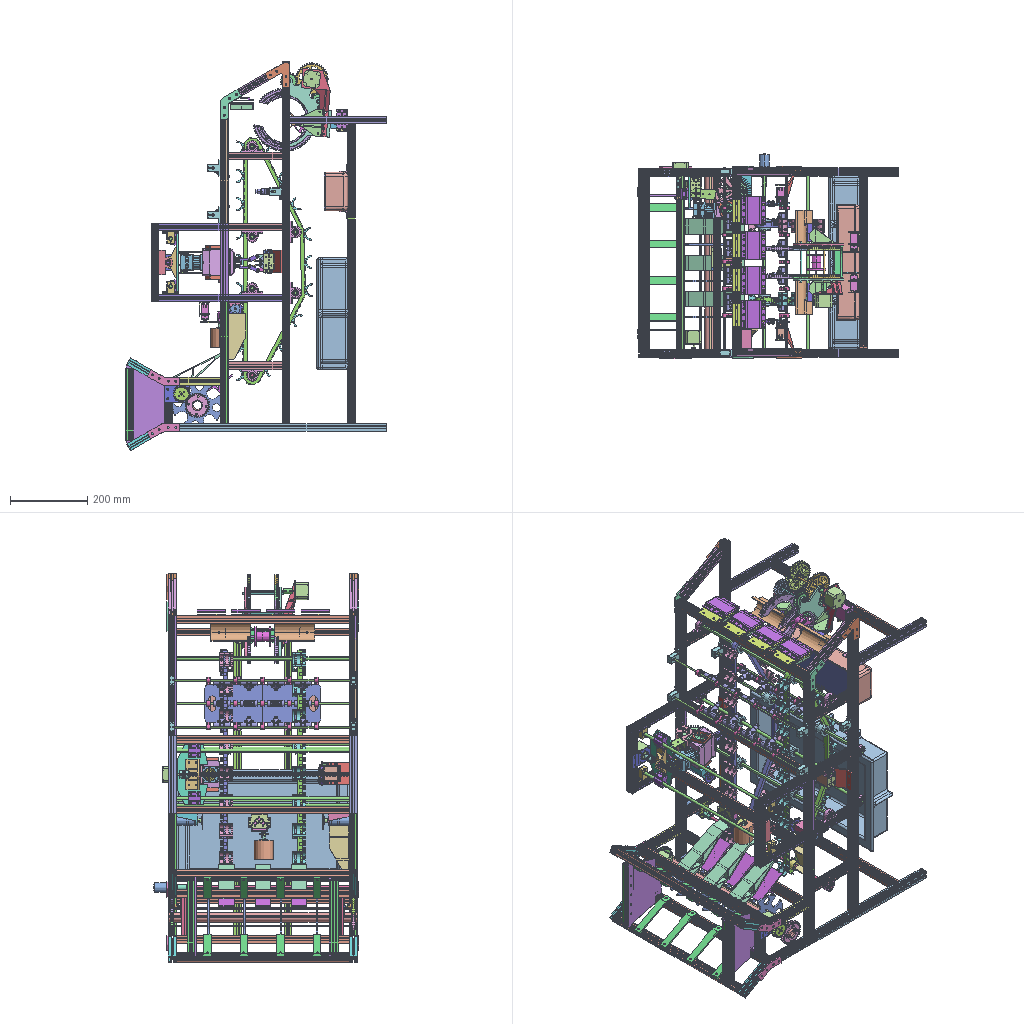Assembly | STEP file | 130 different items | 376 placed | box 676 x 533 x 1010 mm
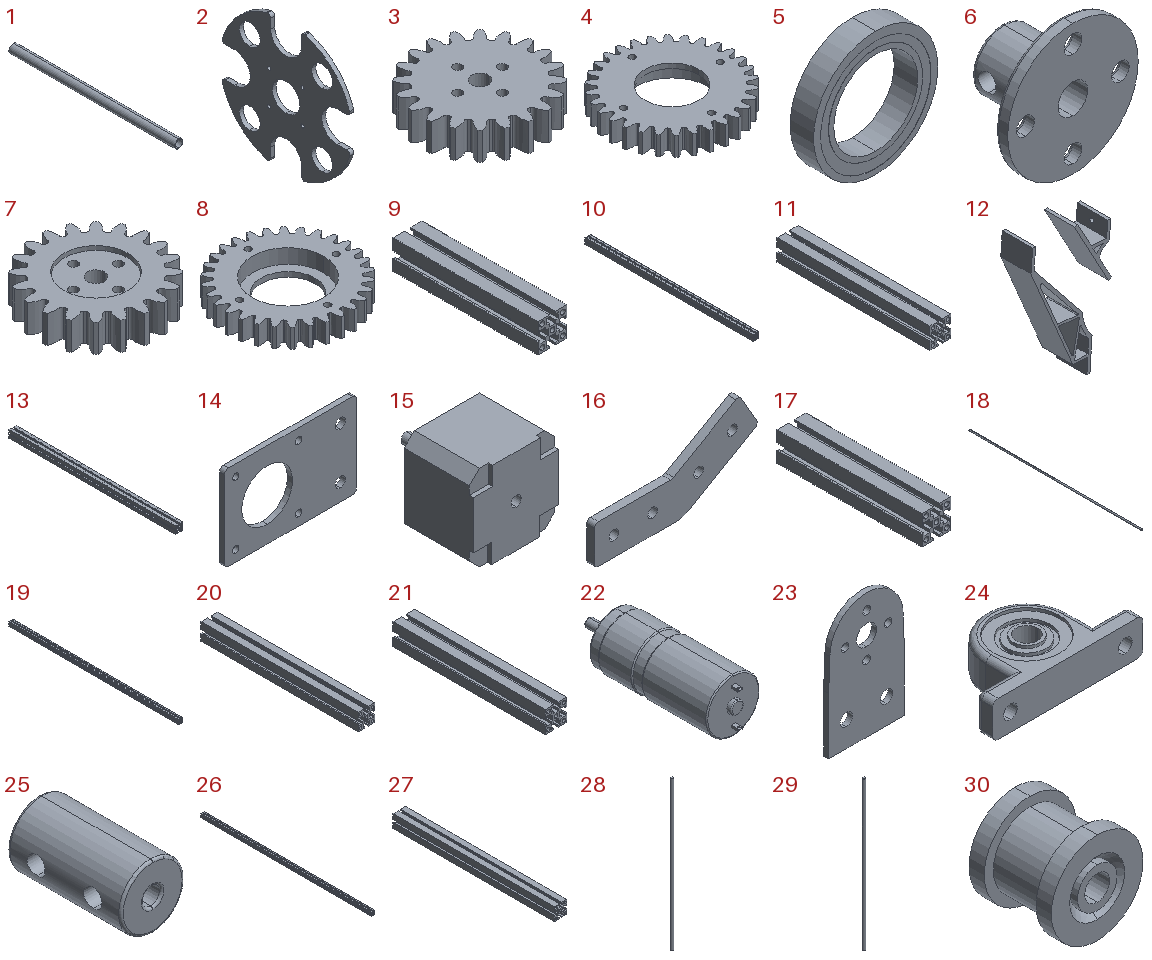Parts list (item | name | quantity | parent item | size | volume):
1 | Central air duct | x1 | - | 25 x 490 x 25 mm | 70811 mm3
2 | Chuck wheel | x4 | - | 4 x 124.659 x 124.659 mm | 32758 mm3
3 | Chuck drive gear | x1 | - | 43.654 x 43.654 x 10 mm | 11238 mm3
4 | Chuck gear | x1 | - | 64 x 63.787 x 10 mm | 17915 mm3
5 | Wheel bearing | x2 | - | 37 x 7 x 37 mm | 4043 mm3
6 | Flange coupling 5 | x2 | - | 22 x 12 x 22 mm | 1230 mm3
7 | Mirror chuck drive gear | x1 | - | 43.654 x 43.654 x 10 mm | 11238 mm3
8 | Mirror chuck gear | x1 | - | 64 x 63.787 x 10 mm | 17915 mm3
9 | 20 aluminium profile longitudinal 1 | x2 | - | 20 x 100 x 20 mm | 17778 mm3
10 | 20 aluminium profile vertical 1 | x2 | - | 20 x 575 x 20 mm | 102223 mm3
11 | 20 aluminium profile vertical 2 | x2 | - | 20 x 145 x 20 mm | 25778 mm3
12 | Chuck limit ring | x3 | - | 105.924 x 40 x 181.464 mm | 85930 mm3
13 | 20 aluminium profile transverse 2 | x10 | - | 20 x 450 x 20 mm | 80001 mm3
14 | 42 stepper aluminium flat bracket | x3 | - | 65 x 2.5 x 42 mm | 5411 mm3
15 | 42 stepper motor 34 | x4 | - | 42 x 54 x 42 mm | 57864 mm3
16 | 150-degree side frame | x4 | - | 83.909 x 4 x 39.268 mm | 6499 mm3
17 | 20 aluminium profile diagonal 1 | x4 | - | 20 x 100 x 20 mm | 17778 mm3
18 | Gear shaft | x4 | - | 4 x 491 x 4 mm | 6170 mm3
19 | 20 aluminium profile longitudinal 1 | x2 | - | 20 x 830 x 20 mm | 147557 mm3
20 | 20 aluminium profile longitudinal 2 | x2 | - | 20 x 186 x 20 mm | 33067 mm3
21 | 20 aluminium profile vertical 1 | x6 | - | 20 x 140 x 20 mm | 24889 mm3
22 | 370 straight motor | x3 | - | 25 x 71.68 x 25 mm | 27082 mm3
23 | Smooth shaft 370 bracket | x1 | - | 30 x 2 x 49.5 mm | 2512 mm3
24 | U-type bearing support 8 | x11 | - | 55 x 30 x 13 mm | 10419 mm3
25 | 48 rigid coupling | x1 | - | 14 x 25 x 14 mm | 2952 mm3
26 | 20 aluminium profile longitudinal 3 | x2 | - | 20 x 940 x 20 mm | 167113 mm3
27 | 20 aluminium profile vertical 2 | x2 | - | 20 x 250 x 20 mm | 44445 mm3
28 | Sprocket 1 shaft | x7 | - | 8 x 8 x 490 mm | 24630 mm3
29 | Sprocket 2 shaft | x1 | - | 8 x 8 x 480 mm | 24127 mm3
30 | B drag chain wheel | x10 | - | 30 x 27 x 30 mm | 13045 mm3
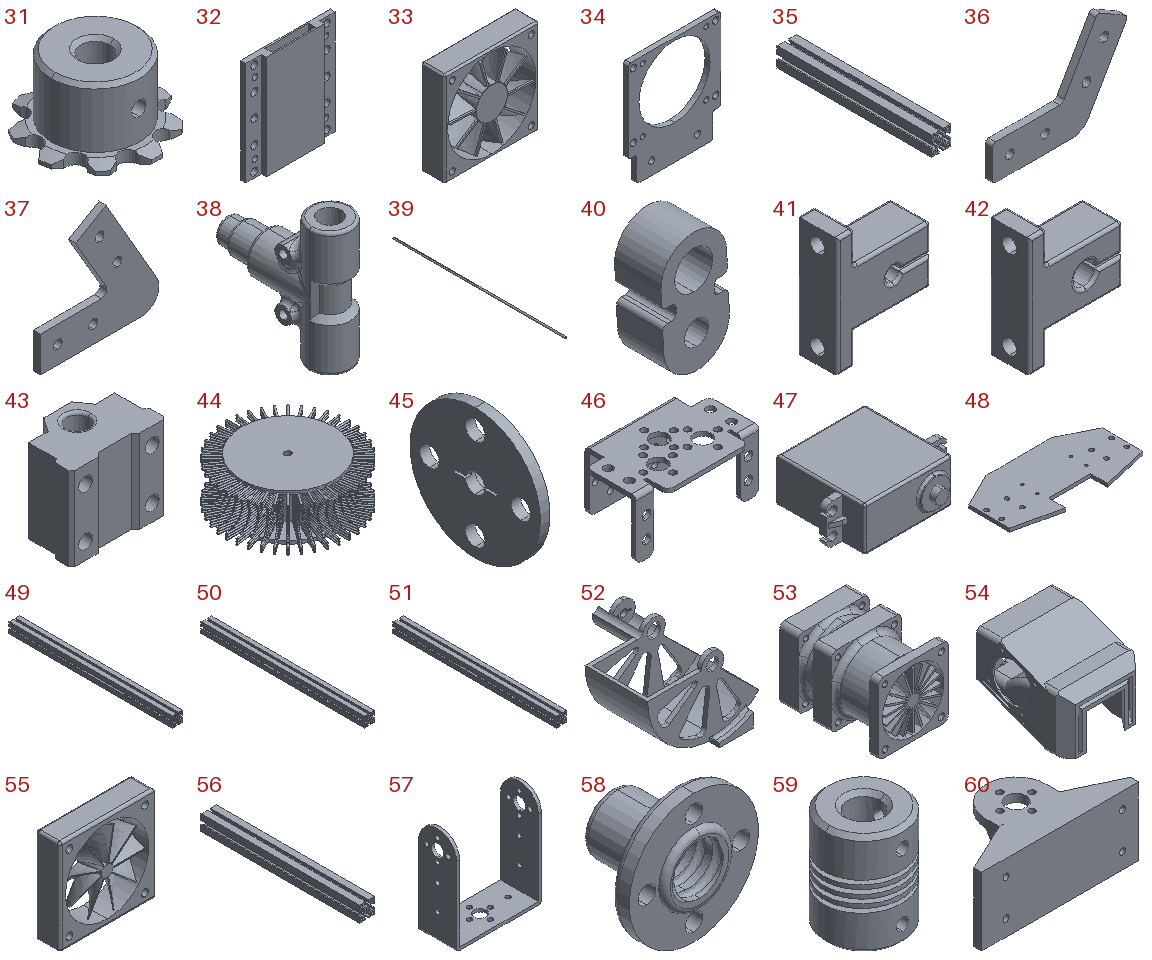31 | Sprocket | x2 | - | 33.749 x 33.304 x 20 mm | 8415 mm3
32 | Heating module 60 low | x4 | - | 63 x 7 x 73 mm | 14494 mm3
33 | Fan 60 | x4 | - | 60 x 15 x 60 mm | 65760 mm3
34 | Drying connection frame | x4 | - | 73 x 4 x 85 mm | 13236 mm3
35 | 20 aluminium profile diagonal 2 | x2 | - | 20 x 160 x 20 mm | 28445 mm3
36 | 120-degree side frame | x2 | - | 76.588 x 4 x 53.909 mm | 6976 mm3
37 | 60-degree side frame | x2 | - | 67.321 x 4 x 64.641 mm | 8608 mm3
38 | Water-bath atomizer head | x12 | - | 15 x 44.7 x 45 mm | 9906 mm3
39 | Cleaning nozzle shaft | x3 | - | 5 x 490 x 5 mm | 9621 mm3
40 | Rotating slot | x15 | - | 14.79 x 10 x 26.2 mm | 2369 mm3
41 | T-type support 5(D) | x6 | - | 32.8 x 14 x 42 mm | 10262 mm3
42 | T-type support 8 | x4 | - | 32.8 x 14 x 42 mm | 9873 mm3
43 | Slider 8 | x2 | - | 34 x 22 x 30 mm | 14928 mm3
44 | Wheel brush | x1 | - | 80 x 80 x 30 mm | 40010 mm3
45 | Large servo disc | x4 | - | 3.5 x 20 x 20 mm | 468.717 mm3
46 | Multifunction bracket | x5 | - | 58 x 37.5 x 28 mm | 5928 mm3
47 | Servo single shaft | x5 | in SW alloy mechanical claw | 55 x 44.5 x 20 mm | 32938 mm3
48 | Sliding plate | x1 | - | 158 x 80 x 4 mm | 40027 mm3
49 | 20 aluminium profile longitudinal 4 | x2 | - | 20 x 310 x 20 mm | 55112 mm3
50 | 20 aluminium profile vertical 6 | x4 | - | 20 x 320 x 20 mm | 56889 mm3
51 | 20 aluminium profile longitudinal 5 | x2 | - | 20 x 316 x 20 mm | 56178 mm3
52 | Peel friction cover | x1 | - | 81.568 x 81 x 58.817 mm | 32383 mm3
53 | Vortex fan 40 | x1 | - | 40 x 56 x 40 mm | 33950 mm3
54 | U-type air nozzle | x1 | - | 70 x 80.5 x 65.068 mm | 54553 mm3
55 | Fan 40 | x2 | - | 40 x 10 x 40 mm | 6606 mm3
56 | 20 aluminium profile longitudinal 6 | x2 | - | 20 x 204 x 20 mm | 36267 mm3
57 | U long bracket | x1 | - | 56 x 25 x 64.5 mm | 8183 mm3
58 | Lead screw nut 8 | x1 | - | 22 x 15 x 22 mm | 1124 mm3
59 | 58 flexible coupling | x1 | - | 19 x 19 x 25 mm | 4870 mm3
60 | Lead screw push block | x1 | - | 78 x 37 x 34 mm | 16349 mm3
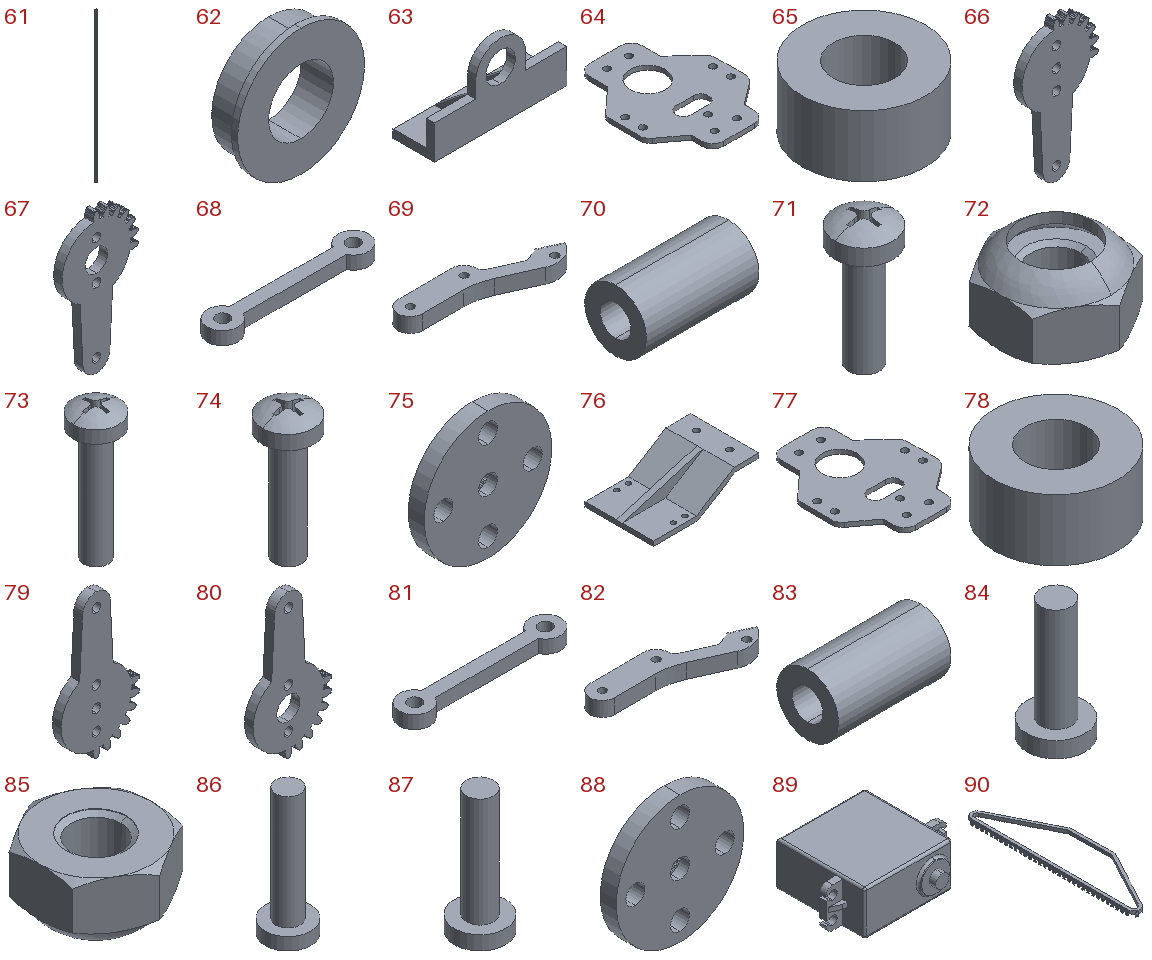61 | Lead screw 1 | x1 | - | 8 x 8 x 450 mm | 16512 mm3
62 | Bearing 814 | x1 | - | 15.6 x 4 x 15.6 mm | 433.486 mm3
63 | Lead screw bearing sleeve | x1 | - | 64.2 x 20 x 36.1 mm | 9790 mm3
64 | Gripper (new)_1 | x1 | in SW alloy mechanical claw | 48 x 61 x 2 mm | 3505 mm3
65 | Small washer_1 | x3 | in SW alloy mechanical claw | 6 x 6 x 3 mm | 63.617 mm3
66 | Claw gear 2 | x1 | in SW alloy mechanical claw | 27.091 x 3 x 49.757 mm | 2108 mm3
67 | Claw gear_1 | x1 | in SW alloy mechanical claw | 27.091 x 3 x 49.757 mm | 1979 mm3
68 | Small crossbar_1 | x2 | in SW alloy mechanical claw | 37 x 7 x 3 mm | 397.481 mm3
69 | Long rod_1 | x2 | in SW alloy mechanical claw | 59.158 x 19.551 x 6 mm | 2724 mm3
70 | Stud_1 | x4 | in SW alloy mechanical claw | 11 x 6 x 6 mm | 233.263 mm3
71 | GB818-M3X10-ZN-4.8_1 | x2 | in SW alloy mechanical claw | 5.6 x 5.6 x 12.376 mm | 116.575 mm3
72 | GB6170-M3 (self-locking)_1 | x9 | in SW alloy mechanical claw | 5.5 x 6.351 x 3.382 mm | 56.307 mm3
73 | GB818-M3X14-ZN-4.8_1 | x6 | in SW alloy mechanical claw | 5.6 x 5.6 x 16.376 mm | 144.849 mm3
74 | GB818-M3X12-ZN-4.8_1 | x1 | in SW alloy mechanical claw | 5.6 x 5.6 x 14.376 mm | 130.712 mm3
75 | Metal main rudder disc | x1 | in SW alloy mechanical claw | 20 x 4.5 x 20 mm | 750.526 mm3
76 | Mechanical claw bracket | x2 | - | 90 x 58 x 24 mm | 23689 mm3
77 | Mirror gripper (new)_1 | x1 | in MirrorSW alloy mechanical claw | 48 x 61 x 2 mm | 3505 mm3
78 | Mirror small washer_1 | x3 | in MirrorSW alloy mechanical claw | 6 x 6 x 3 mm | 63.617 mm3
79 | Mirror claw gear 2 | x1 | in MirrorSW alloy mechanical claw | 27.091 x 3 x 49.757 mm | 2108 mm3
80 | Mirror claw gear_1 | x1 | in MirrorSW alloy mechanical claw | 27.091 x 3 x 49.757 mm | 1979 mm3
81 | Mirror small crossbar_1 | x2 | in MirrorSW alloy mechanical claw | 37 x 7 x 3 mm | 397.481 mm3
82 | Mirror long rod_1 | x2 | in MirrorSW alloy mechanical claw | 59.158 x 19.551 x 6 mm | 2724 mm3
83 | Mirror stud_1 | x4 | in MirrorSW alloy mechanical claw | 11 x 6 x 6 mm | 233.263 mm3
84 | MirrorGB818-M3X10-ZN-4.8_1 | x2 | in MirrorSW alloy mechanical claw | 5.6 x 5.6 x 12.376 mm | 116.575 mm3
85 | MirrorGB6170-M3 (self-locking)_1 | x9 | in MirrorSW alloy mechanical claw | 5.5 x 6.351 x 3.382 mm | 56.307 mm3
86 | MirrorGB818-M3X14-ZN-4.8_1 | x6 | in MirrorSW alloy mechanical claw | 5.6 x 5.6 x 16.376 mm | 144.849 mm3
87 | MirrorGB818-M3X12-ZN-4.8_1 | x1 | in MirrorSW alloy mechanical claw | 5.6 x 5.6 x 14.376 mm | 130.712 mm3
88 | Mirror metal main rudder disc | x1 | in MirrorSW alloy mechanical claw | 20 x 4.5 x 20 mm | 750.526 mm3
89 | Mirror servo single shaft | x1 | in MirrorSW alloy mechanical claw | 55 x 44.5 x 20 mm | 32938 mm3
90 | Belt 1 | x1 | - | 163.112 x 641.3 x 20 mm | 175468 mm3
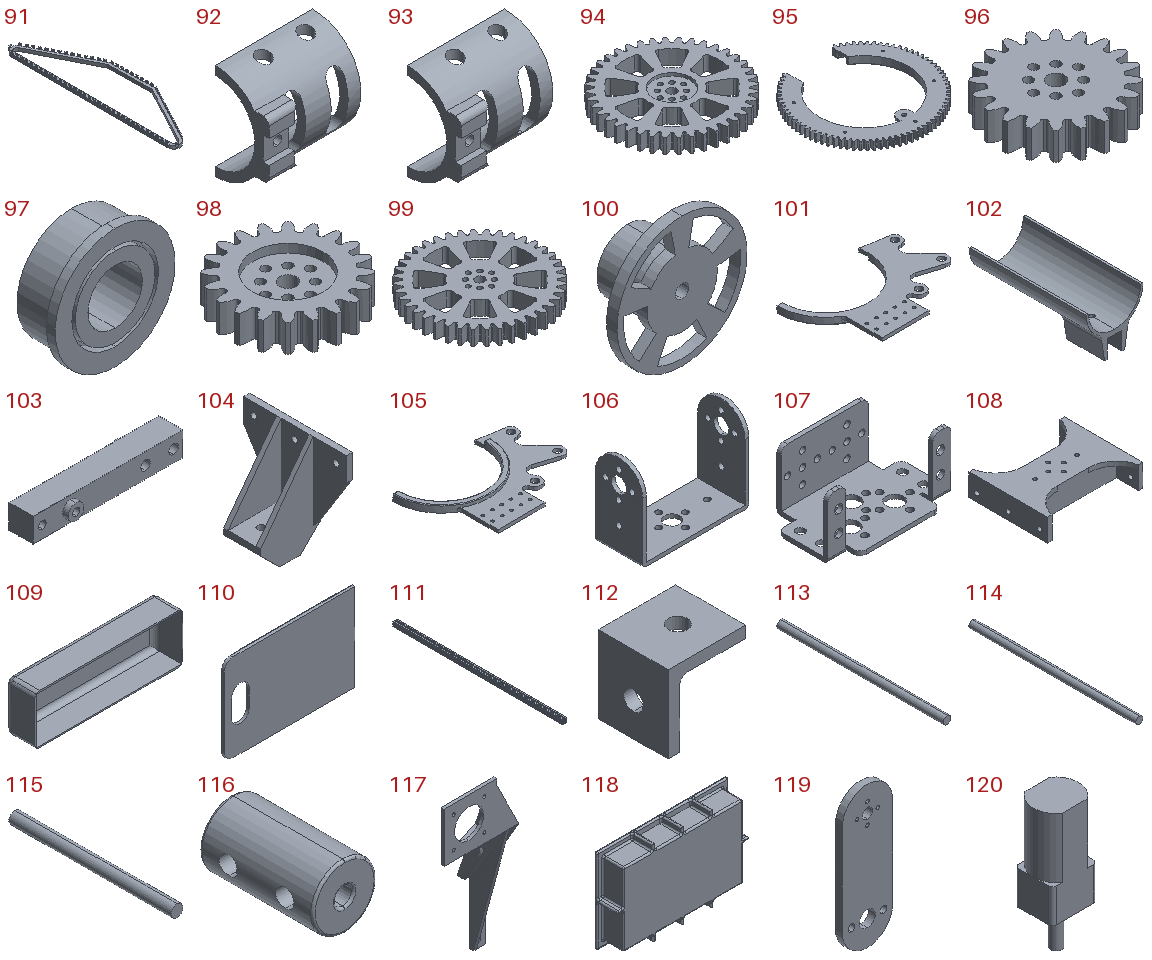91 | Mirror belt 1 | x1 | - | 163.112 x 641.3 x 20 mm | 175468 mm3
92 | Chain frame | x18 | - | 34.45 x 19 x 34 mm | 4420 mm3
93 | Mirror chain frame | x18 | - | 34.45 x 19 x 34 mm | 4420 mm3
94 | FD gear 40 | x1 | - | 83.847 x 83.847 x 10 mm | 32005 mm3
95 | Packing half-gear | x2 | - | 163.929 x 156.763 x 10 mm | 60681 mm3
96 | FD gear 20 | x2 | - | 43.654 x 43.654 x 10 mm | 10262 mm3
97 | Flange bearing 5104 | x6 | - | 11 x 4 x 11 mm | 233.729 mm3
98 | MirrorFD gear 20 | x2 | - | 43.654 x 43.654 x 10 mm | 10262 mm3
99 | MirrorFD gear 40 | x1 | - | 83.847 x 83.847 x 10 mm | 32005 mm3
100 | Packing half-frame | x2 | - | 50 x 21 x 50 mm | 8229 mm3
101 | Half-gear guide groove revised | x1 | - | 193.874 x 133 x 10.2 mm | 53575 mm3
102 | Weighing slot | x2 | - | 50 x 103.5 x 42.709 mm | 22376 mm3
103 | Weighing module | x2 | - | 80 x 18.8 x 12.8 mm | 12498 mm3
104 | Weighing fixed frame | x2 | - | 40 x 70 x 65.291 mm | 23281 mm3
105 | Mirror half-gear guide groove revised | x1 | - | 193.874 x 133 x 10.2 mm | 53575 mm3
106 | U short bracket | x1 | - | 56 x 25 x 44.5 mm | 6211 mm3
107 | Mirror multifunction bracket | x1 | - | 58 x 37.5 x 28 mm | 5928 mm3
108 | Servo connection frame | x1 | - | 85 x 70 x 20 mm | 29316 mm3
109 | 301 water tank | x1 | - | 300 x 58 x 100 mm | 214812 mm3
110 | 301 water tank cover | x2 | - | 150 x 6 x 100 mm | 46035 mm3
111 | 20 aluminium profile longitudinal 7 | x2 | - | 20 x 778 x 20 mm | 138312 mm3
112 | 20 angle bracket flat | x8 | - | 20 x 18 x 20 mm | 1896 mm3
113 | Rear shaft short | x2 | - | 5 x 106 x 5 mm | 2081 mm3
114 | Rear shaft long | x1 | - | 5 x 116 x 5 mm | 2278 mm3
115 | Rear winding spool | x1 | - | 5 x 68 x 5 mm | 1335 mm3
116 | 55 rigid coupling | x1 | - | 14 x 25 x 14 mm | 3316 mm3
117 | Rear stepper bracket | x1 | - | 75 x 37 x 171.474 mm | 24600 mm3
118 | Basket 1 | x1 | - | 450 x 80 x 290 mm | 2294003 mm3
119 | Dial wheel bracket | x1 | - | 22 x 3 x 62 mm | 3552 mm3
120 | N201 | x2 | - | 12 x 10 x 35 mm | 2772 mm3
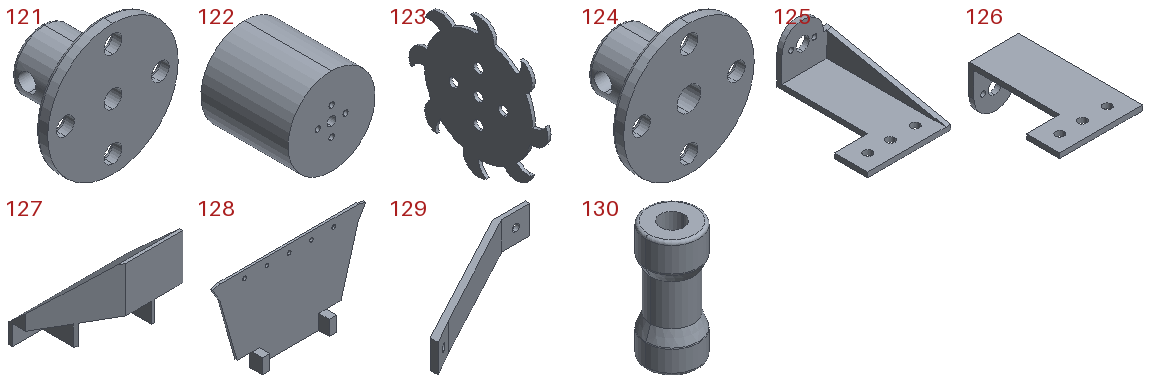121 | Flange coupling 3 | x1 | - | 22 x 12 x 22 mm | 1380 mm3
122 | Dial wheel | x1 | - | 50 x 50 x 50 mm | 41621 mm3
123 | Cutting knife | x2 | - | 1 x 45 x 45 mm | 1128 mm3
124 | Flange coupling 4 | x2 | - | 22 x 12 x 22 mm | 1314 mm3
125 | Cutting motor bracket | x1 | - | 50 x 74.62 x 30.335 mm | 11204 mm3
126 | Mirror cutting motor bracket | x1 | - | 50 x 74.62 x 30.335 mm | 11204 mm3
127 | Top plate | x1 | - | 120 x 53 x 65 mm | 56002 mm3
128 | Bin side panel | x2 | - | 206.163 x 17 x 120.782 mm | 62585 mm3
129 | Front frame | x8 | - | 118.103 x 56.081 x 20 mm | 10734 mm3
130 | Brass coupling 3-4 | x1 | - | 9 x 9 x 20 mm | 848.219 mm3
Placements (level | parent | child | x y z in mm | rotation matrix by rows), first 264 of 378 lines:
1 | subassembly 2 | Central air duct | -58.969 -295.759 -262.917 | 0.04399 0 -0.999 0 1 0 0.999 0 0.04399
1 | subassembly 2 | Chuck wheel | -58.969 -152.758 -262.917 | 0 0.6192 0.7852 -1 0 0 0 -0.7852 0.6192
1 | subassembly 2 | Chuck drive gear | -99.969 -526.259 -233.434 | -0.6467 -0.7627 0 0 0 -1 0.7627 -0.6467 -0
1 | subassembly 2 | Chuck gear | -58.969 -526.259 -262.917 | -0.02036 0.9998 0 0 0 -1 -0.9998 -0.02036 -0
1 | subassembly 2 | Wheel bearing | -58.969 -530.259 -262.917 | 1 0 0 0 1 0 0 0 1
1 | subassembly 2 | Flange coupling 5 | -99.969 -527.759 -233.434 | 0.6467 0 0.7627 0 1 0 -0.7627 0 0.6467
1 | subassembly 2 | Chuck wheel | -58.969 -438.759 -262.917 | 0 0.6192 -0.7852 1 0 0 0 -0.7852 -0.6192
1 | subassembly 2 | Mirror chuck drive gear | -99.969 -65.258 -233.434 | -0.6467 -0.7627 0 0 0 -1 0.7627 -0.6467 -0
1 | subassembly 2 | Flange coupling 5 | -99.969 -63.758 -233.434 | 0.6467 0 -0.7627 0 -1 0 -0.7627 0 -0.6467
1 | subassembly 2 | Mirror chuck gear | -58.969 -65.258 -262.917 | -0.02036 0.9998 0 0 0 -1 -0.9998 -0.02036 -0
1 | subassembly 2 | Wheel bearing | -58.969 -61.258 -262.917 | -1 0 0 0 -1 0 0 0 1
1 | subassembly 2 | 20 aluminium profile longitudinal 1 | -133.969 -495.759 -210.171 | 1 0 0 0 0 1 0 -1 -0
1 | subassembly 2 | 20 aluminium profile vertical 1 | -143.969 -60.758 -320.171 | 0 1 0 -1 0 0 0 0 1
1 | subassembly 2 | 20 aluminium profile vertical 2 | -143.969 -60.758 -200.171 | 0 1 0 -1 0 0 0 0 1
1 | subassembly 2 | Chuck limit ring | -59.043 -409.759 -261.81 | 0.06683 0 0.9978 0 1 0 -0.9978 0 0.06683
1 | subassembly 2 | 20 aluminium profile transverse 2 | -228.411 -520.759 -153.429 | 0.866 0 0.5 0 1 0 -0.5 0 0.866
1 | subassembly 2 | Chuck limit ring | -59.043 -221.758 -261.81 | 0.06683 0 0.9978 0 1 0 -0.9978 0 0.06683
1 | subassembly 2 | 42 stepper aluminium flat bracket | -111.469 -507.009 -233.434 | -1 0 0 0 -1 0 0 0 1
1 | subassembly 2 | 42 stepper motor 34 | -99.969 -471.759 -233.434 | 1 0 0 0 -1 0 0 0 -1
1 | subassembly 2 | 150-degree side frame | -144.773 -46.758 -330.171 | 0.866 0 0.5 0 -1 0 0.5 0 -0.866
1 | subassembly 2 | 150-degree side frame | -144.773 -50.758 -190.171 | 0.866 0 0.5 0 1 0 -0.5 0 0.866
1 | subassembly 2 | 20 aluminium profile diagonal 1 | -237.071 -60.758 -371.913 | 0 0.866 -0.5 -1 0 0 0 0.5 0.866
1 | subassembly 2 | 20 aluminium profile diagonal 1 | -237.071 -60.758 -148.429 | 0 0.866 0.5 -1 0 0 0 -0.5 0.866
1 | subassembly 2 | 20 aluminium profile transverse 2 | -133.969 -520.759 -320.171 | 1 0 0 0 1 0 0 0 1
1 | subassembly 2 | 20 aluminium profile transverse 2 | -228.411 -520.759 -366.913 | 0.866 0 -0.5 0 1 0 0.5 0 0.866
1 | subassembly 2 | 20 aluminium profile vertical 2 | -143.969 -530.759 -200.171 | 0 1 0 1 0 0 0 0 -1
1 | subassembly 2 | 42 stepper aluminium flat bracket | -111.469 -84.508 -233.434 | -1 0 0 0 1 0 0 0 -1
1 | subassembly 2 | 42 stepper motor 34 | -99.969 -119.758 -233.434 | 1 0 0 0 1 0 0 0 1
1 | subassembly 2 | 20 aluminium profile vertical 1 | -143.969 -530.759 -320.171 | 0 1 0 1 0 0 0 0 -1
1 | subassembly 2 | 20 aluminium profile longitudinal 1 | -133.969 -95.758 -210.171 | 1 0 0 0 0 1 0 -1 0
1 | subassembly 2 | 150-degree side frame | -144.773 -544.759 -190.171 | 0.866 0 0.5 0 1 0 -0.5 0 0.866
1 | subassembly 2 | 20 aluminium profile diagonal 1 | -237.071 -530.759 -148.429 | 0 0.866 -0.5 1 0 0 0 -0.5 -0.866
1 | subassembly 2 | 150-degree side frame | -144.773 -540.759 -330.171 | 0.866 0 0.5 0 -1 0 0.5 0 -0.866
1 | subassembly 2 | 20 aluminium profile diagonal 1 | -237.071 -530.759 -371.913 | 0 0.866 0.5 1 0 0 0 0.5 -0.866
1 | subassembly 2 | 20 aluminium profile transverse 2 | -133.969 -520.759 -200.171 | 1 0 0 0 1 0 0 0 1
1 | subassembly 2 | Gear shaft | -56.269 -541.259 -240.076 | -0.5288 0 0.8488 0 1 0 -0.8488 0 -0.5288
1 | subassembly 2 | Gear shaft | -81.81 -541.259 -260.216 | 0.8488 0 0.5288 0 1 0 -0.5288 0 0.8488
1 | subassembly 2 | Gear shaft | -61.669 -541.259 -285.758 | 0.5288 0 -0.8488 0 1 0 0.8488 0 0.5288
1 | subassembly 2 | Gear shaft | -36.128 -541.259 -265.617 | -0.8488 0 -0.5288 0 1 0 0.5288 0 -0.8488
1 | subassembly 2 | Chuck wheel | -58.969 -246.758 -262.917 | 0 0.6192 0.7852 -1 0 0 0 -0.7852 0.6192
1 | subassembly 2 | Chuck wheel | -58.969 -344.759 -262.917 | 0 0.6192 -0.7852 1 0 0 0 -0.7852 -0.6192
1 | subassembly 2 | Chuck limit ring | -59.043 -315.759 -261.81 | 0.06683 0 0.9978 0 1 0 -0.9978 0 0.06683
1 | subassembly 2 | 20 aluminium profile longitudinal 1 | 11.031 -60.758 519.829 | 0 0 1 -1 0 0 0 -1 0
1 | subassembly 2 | 20 aluminium profile transverse 2 | 11.019 -70.758 -216.604 | -1 0 0 0 -1 0 0 0 1
1 | subassembly 2 | 20 aluminium profile longitudinal 2 | -234.751 -109.758 -167.09 | -1 0 0 0 0 -1 0 -1 -0
1 | subassembly 2 | 20 aluminium profile vertical 1 | 161.031 -60.758 -160.171 | 0 -1 0 1 0 0 0 0 1
1 | subassembly 2 | 370 straight motor | 83.531 -14.959 -185.171 | 1 0 0 0 -1 0 0 0 -1
1 | subassembly 2 | Smooth shaft 370 bracket | 83.531 -70.758 -160.171 | 1 0 0 0 -1 0 0 0 -1
1 | subassembly 2 | U-type bearing support 8 | 111.031 -524.759 -170.171 | -1 0 0 0 0 -1 0 -1 -0
1 | subassembly 2 | 48 rigid coupling | 83.531 -86.258 -185.171 | -1 0 0 0 -1 0 0 0 1
1 | subassembly 2 | 20 aluminium profile longitudinal 1 | 11.031 -530.759 519.829 | 0 0 -1 1 0 0 0 -1 -0
1 | subassembly 2 | 20 aluminium profile vertical 1 | 161.031 -530.759 -160.171 | 0 -1 0 -1 0 0 0 0 -1
1 | subassembly 2 | 20 aluminium profile longitudinal 3 | 171.031 -60.758 -310.171 | 1 0 0 0 0 -1 0 1 0
1 | subassembly 2 | 20 aluminium profile vertical 2 | 181.031 -60.758 477.829 | 0 1 0 -1 0 0 0 0 1
1 | subassembly 2 | U-type bearing support 8 | 111.031 -54.258 189.829 | -1 0 0 0 0 -1 0 -1 -0
1 | subassembly 2 | 20 aluminium profile longitudinal 3 | 171.031 -530.759 -310.171 | 1 0 0 0 0 -1 0 1 -0
1 | subassembly 2 | 20 aluminium profile vertical 2 | 181.031 -530.759 477.829 | 0 1 0 1 0 0 0 0 -1
1 | subassembly 2 | U-type bearing support 8 | 111.031 -524.259 189.829 | -1 0 0 0 0 -1 0 -1 0
1 | subassembly 2 | 20 aluminium profile longitudinal 2 | -234.751 -481.759 -167.09 | -1 0 0 0 0 -1 0 -1 0
1 | subassembly 2 | 20 aluminium profile transverse 2 | 11.031 -520.759 509.829 | 1 0 0 0 1 0 0 0 1
1 | subassembly 2 | Sprocket 1 shaft | 83.531 -50.758 174.829 | -0.6621 0.7494 0 0 0 -1 -0.7494 -0.6621 -0
1 | subassembly 2 | Sprocket 2 shaft | 83.531 -60.758 -185.171 | 0.9963 -0.08586 0 0 0 -1 0.08586 0.9963 0
1 | subassembly 2 | B drag chain wheel | 83.531 -211.398 174.829 | 0.9904 0 -0.1384 0 1 0 0.1384 0 0.9904
1 | subassembly 2 | Sprocket | 83.531 -199.358 -185.171 | -0.6415 -0.7671 0 0 0 1 -0.7671 0.6415 -0
1 | subassembly 2 | B drag chain wheel | 83.531 -380.119 174.829 | 0.9904 0 0.1384 0 -1 0 0.1384 0 -0.9904
1 | subassembly 2 | Sprocket | 83.531 -392.159 -185.171 | 0.6415 -0.7671 0 0 0 -1 0.7671 0.6415 -0
1 | subassembly 2 | Heating module 60 low | 56.031 -162.258 534.829 | 1 0 0 0 0 1 0 -1 0
1 | subassembly 2 | Fan 60 | 56.031 -162.258 504.829 | -1 0 0 0 0 1 0 1 0
1 | subassembly 2 | Fan 60 | 56.031 -252.258 504.829 | -1 0 0 0 0 1 0 1 0
1 | subassembly 2 | Fan 60 | 56.031 -342.259 504.829 | -1 0 0 0 0 1 0 1 0
1 | subassembly 2 | Fan 60 | 56.031 -432.259 504.829 | -1 0 0 0 0 1 0 1 0
1 | subassembly 2 | Heating module 60 low | 56.031 -252.258 534.829 | 1 0 0 0 0 1 0 -1 0
1 | subassembly 2 | Heating module 60 low | 56.031 -342.259 534.829 | 1 0 0 0 0 1 0 -1 0
1 | subassembly 2 | Heating module 60 low | 56.031 -432.259 534.829 | 1 0 0 0 0 1 0 -1 0
1 | subassembly 2 | Drying connection frame | 43.531 -162.258 523.829 | 0 0 1 -1 0 0 0 -1 -0
1 | subassembly 2 | Drying connection frame | 43.531 -252.258 523.829 | 0 0 1 -1 0 0 0 -1 -0
1 | subassembly 2 | Drying connection frame | 43.531 -342.259 523.829 | 0 0 1 -1 0 0 0 -1 -0
1 | subassembly 2 | Drying connection frame | 43.531 -432.259 523.829 | 0 0 1 -1 0 0 0 -1 -0
1 | subassembly 2 | 20 aluminium profile diagonal 2 | 154.595 -60.758 608.489 | 0.5 -0.866 0 0 0 1 -0.866 -0.5 -0
1 | subassembly 2 | 120-degree side frame | 21.031 -50.758 519.829 | -0.866 0 0.5 0 1 0 -0.5 0 -0.866
1 | subassembly 2 | 60-degree side frame | 161.031 -50.758 600.658 | 0 0 -1 0 1 0 1 0 0
1 | subassembly 2 | 60-degree side frame | 161.031 -544.759 600.658 | 0 0 -1 0 1 0 1 0 0
1 | subassembly 2 | 20 aluminium profile diagonal 2 | 154.595 -530.759 608.489 | 0.5 -0.866 0 0 0 1 -0.866 -0.5 0
1 | subassembly 2 | 120-degree side frame | 21.031 -544.759 519.829 | -0.866 0 0.5 0 1 0 -0.5 0 -0.866
1 | subassembly 2 | Water-bath atomizer head | -8.282 -189.529 347.339 | -0.5 0.866 0 0 0 -1 -0.866 -0.5 -0
1 | subassembly 2 | Water-bath atomizer head | -8.282 -259.529 347.339 | -0.5 0.866 0 0 0 -1 -0.866 -0.5 -0
1 | subassembly 2 | Water-bath atomizer head | -8.282 -329.529 347.339 | -0.5 0.866 0 0 0 -1 -0.866 -0.5 -0
1 | subassembly 2 | Water-bath atomizer head | -8.282 -399.529 347.339 | -0.5 0.866 0 0 0 -1 -0.866 -0.5 -0
1 | subassembly 2 | Cleaning nozzle shaft | -18.969 -540.759 352.829 | 0.9967 0 -0.08123 0 1 0 0.08123 0 0.9967
1 | subassembly 2 | Rotating slot | -18.969 -154.529 352.829 | -0.5 0 0.866 0 1 0 -0.866 0 -0.5
1 | subassembly 2 | 20 aluminium profile vertical 1 | 161.031 -60.758 199.829 | 0 -1 0 1 0 0 0 0 1
1 | subassembly 2 | Rotating slot | -18.969 -224.529 352.829 | -0.5 0 0.866 0 1 0 -0.866 0 -0.5
1 | subassembly 2 | Rotating slot | -18.969 -294.529 352.829 | -0.5 0 0.866 0 1 0 -0.866 0 -0.5
1 | subassembly 2 | Rotating slot | -18.969 -364.529 352.829 | -0.5 0 0.866 0 1 0 -0.866 0 -0.5
1 | subassembly 2 | Rotating slot | -18.969 -434.529 352.829 | -0.5 0 0.866 0 1 0 -0.866 0 -0.5
1 | subassembly 2 | Cleaning nozzle shaft | -18.969 -540.759 230.829 | 0.9967 0 0.08123 0 1 0 -0.08123 0 0.9967
1 | subassembly 2 | Rotating slot | -18.969 -154.529 230.829 | -0.5 0 0.866 0 -1 0 0.866 0 0.5
1 | subassembly 2 | Water-bath atomizer head | -8.282 -189.529 236.318 | 0.5 0.866 0 0 0 -1 -0.866 0.5 0
1 | subassembly 2 | Rotating slot | -18.969 -224.529 230.829 | -0.5 0 0.866 0 -1 0 0.866 0 0.5
1 | subassembly 2 | Water-bath atomizer head | -8.282 -259.529 236.318 | 0.5 0.866 0 0 0 -1 -0.866 0.5 0
1 | subassembly 2 | Rotating slot | -18.969 -294.529 230.829 | -0.5 0 0.866 0 -1 0 0.866 0 0.5
1 | subassembly 2 | Water-bath atomizer head | -8.282 -329.529 236.318 | 0.5 0.866 0 0 0 -1 -0.866 0.5 0
1 | subassembly 2 | Rotating slot | -18.969 -364.529 230.829 | -0.5 0 0.866 0 -1 0 0.866 0 0.5
1 | subassembly 2 | Water-bath atomizer head | -8.282 -399.529 236.318 | 0.5 0.866 0 0 0 -1 -0.866 0.5 0
1 | subassembly 2 | Rotating slot | -18.969 -434.529 230.829 | -0.5 0 0.866 0 -1 0 0.866 0 0.5
1 | subassembly 2 | 20 aluminium profile vertical 1 | 161.031 -60.758 383.829 | 0 -1 0 1 0 0 0 0 1
1 | subassembly 2 | U-type bearing support 8 | 111.031 -537.259 393.829 | -1 0 0 0 0 1 0 1 0
1 | subassembly 2 | B drag chain wheel | 83.531 -380.119 408.829 | 0.9904 0 -0.1384 0 -1 0 -0.1384 0 -0.9904
1 | subassembly 2 | Sprocket 1 shaft | 83.531 -540.759 408.829 | -0.6621 0.7494 0 0 0 1 0.7494 0.6621 0
1 | subassembly 2 | B drag chain wheel | 83.531 -211.398 408.829 | 0.9904 0 0.1384 0 1 0 -0.1384 0 0.9904
1 | subassembly 2 | U-type bearing support 8 | 111.031 -67.258 393.829 | -1 0 0 0 0 1 0 1 0
1 | subassembly 2 | T-type support 5(D) | 1.031 -53.258 352.829 | -1 0 0 0 -1 0 0 0 1
1 | subassembly 2 | T-type support 5(D) | 1.031 -524.259 352.829 | -1 0 0 0 -1 0 0 0 1
1 | subassembly 2 | 20 aluminium profile vertical 1 | 161.031 -530.759 199.829 | 0 -1 0 -1 0 0 0 0 -1
1 | subassembly 2 | T-type support 5(D) | 1.031 -538.259 230.829 | -1 0 0 0 1 0 0 0 -1
1 | subassembly 2 | T-type support 5(D) | 1.031 -67.258 230.829 | -1 0 0 0 1 0 0 0 -1
1 | subassembly 2 | 20 aluminium profile vertical 1 | 161.031 -530.759 383.829 | 0 -1 0 -1 0 0 0 0 -1
1 | subassembly 2 | T-type support 5(D) | 161.031 -53.258 291.829 | -1 0 0 0 -1 0 0 0 1
1 | subassembly 2 | Cleaning nozzle shaft | 141.031 -540.759 291.829 | 0.9967 0 -0.08123 0 1 0 0.08123 0 0.9967
1 | subassembly 2 | Rotating slot | 141.031 -154.529 291.829 | 0.04908 0 -0.9988 0 1 0 0.9988 0 0.04908
1 | subassembly 2 | Water-bath atomizer head | 129.017 -189.529 291.829 | 0 -1 0 0 0 -1 1 0 -0
1 | subassembly 2 | Rotating slot | 141.031 -224.529 291.829 | 0.04908 0 -0.9988 0 1 0 0.9988 0 0.04908
1 | subassembly 2 | Rotating slot | 141.031 -294.529 291.829 | 0.04908 0 -0.9988 0 1 0 0.9988 0 0.04908
1 | subassembly 2 | Rotating slot | 141.031 -364.529 291.829 | 0.04908 0 -0.9988 0 1 0 0.9988 0 0.04908
1 | subassembly 2 | Rotating slot | 141.031 -434.529 291.829 | 0.04908 0 -0.9988 0 1 0 0.9988 0 0.04908
1 | subassembly 2 | Water-bath atomizer head | 129.017 -259.529 291.829 | 0 -1 0 0 0 -1 1 0 -0
1 | subassembly 2 | Water-bath atomizer head | 129.017 -329.529 291.829 | 0 -1 0 0 0 -1 1 0 -0
1 | subassembly 2 | Water-bath atomizer head | 129.017 -399.529 291.829 | 0 -1 0 0 0 -1 1 0 -0
1 | subassembly 2 | T-type support 5(D) | 161.031 -524.259 291.829 | -1 0 0 0 -1 0 0 0 1
1 | subassembly 2 | T-type support 8 | -127.969 -53.258 189.829 | 0 0 -1 0 -1 0 -1 0 0
1 | subassembly 2 | T-type support 8 | -127.969 -53.258 25.829 | 0 0 1 0 -1 0 1 0 -0
1 | subassembly 2 | Sprocket 1 shaft | -127.969 -50.758 169.829 | -0.6621 0.7494 0 0 0 -1 -0.7494 -0.6621 -0
1 | subassembly 2 | Sprocket 1 shaft | -127.969 -50.758 45.829 | -0.4085 0.9128 0 0 0 -1 -0.9128 -0.4085 -0
1 | subassembly 2 | Slider 8 | -112.969 -133.258 169.829 | 0 -1 0 0 0 1 -1 0 0
1 | subassembly 2 | Slider 8 | -112.969 -133.258 45.829 | 0 -1 0 0 0 1 -1 0 0
1 | subassembly 2 | Wheel brush | 9.091 -110.345 92.829 | 0.8642 -0.5032 0 0.5032 0.8642 0 0 0 1
1 | subassembly 2 | Large servo disc | -93.969 -116.758 81.829 | 0 -0.9584 0.2853 0 -0.2853 -0.9584 1 0 -0
1 | subassembly 2 | Multifunction bracket | -106.969 -106.964 107.508 | 0 0 -1 -1 0 0 0 1 -0
1 | subassembly 2 | Servo single shaft | -83.969 -105.758 107.829 | 0 0 -1 -1 0 0 0 1 -0
1 | subassembly 2 | Sliding plate | -110.969 -113.258 107.829 | 0 0 -1 0 1 0 1 0 0
1 | subassembly 2 | 20 aluminium profile longitudinal 4 | 11.031 -60.758 519.829 | -1 0 0 0 0 -1 0 -1 -0
1 | subassembly 2 | 20 aluminium profile vertical 6 | -158.969 -60.758 199.829 | 0 1 0 -1 0 0 0 0 1
1 | subassembly 2 | 20 aluminium profile vertical 6 | -158.969 -60.758 15.829 | 0 1 0 -1 0 0 0 0 1
1 | subassembly 2 | U-type bearing support 8 | 111.031 -67.258 25.829 | -1 0 0 0 0 1 0 1 0
1 | subassembly 2 | Sprocket 1 shaft | 83.531 -540.759 40.829 | -0.6621 0.7494 0 0 0 1 0.7494 0.6621 0
1 | subassembly 2 | U-type bearing support 8 | 111.031 -537.259 25.829 | -1 0 0 0 0 1 0 1 0
1 | subassembly 2 | B drag chain wheel | 83.531 -380.119 40.829 | 0.9904 0 -0.1384 0 -1 0 -0.1384 0 -0.9904
1 | subassembly 2 | B drag chain wheel | 83.531 -211.398 40.829 | 0.9904 0 0.1384 0 1 0 -0.1384 0 0.9904
1 | subassembly 2 | 20 aluminium profile vertical 6 | -158.969 -530.759 15.829 | 0 1 0 1 0 0 0 0 -1
1 | subassembly 2 | 20 aluminium profile vertical 6 | -158.969 -530.759 199.829 | 0 1 0 1 0 0 0 0 -1
1 | subassembly 2 | 20 aluminium profile longitudinal 4 | 11.031 -530.759 519.829 | -1 0 0 0 0 -1 0 -1 0
1 | subassembly 2 | T-type support 8 | -127.969 -524.259 189.829 | 0 0 -1 0 -1 0 -1 0 0
1 | subassembly 2 | T-type support 8 | -127.969 -524.259 25.829 | 0 0 1 0 -1 0 1 0 -0
1 | subassembly 2 | 20 aluminium profile longitudinal 5 | 11.031 -60.758 5.829 | -1 0 0 0 0 -1 0 -1 -0
1 | subassembly 2 | Peel friction cover | 9.091 -110.345 107.829 | -0.05917 0 0.9982 -0.9982 0 -0.05917 0 -1 -0
1 | subassembly 2 | Vortex fan 40 | -44.52 -161.331 107.829 | 0.05917 -0.9982 0 0.9982 0.05917 0 0 0 1
1 | subassembly 2 | U-type air nozzle | 21.106 -161.145 107.829 | 0 -0.9982 -0.05917 0 0.05917 -0.9982 1 0 -0
1 | subassembly 2 | Fan 40 | -13.14 -157.091 141.829 | 0.9511 0 0.3089 0.3089 0 -0.9511 0 1 -0
1 | subassembly 2 | Fan 40 | -13.14 -157.091 63.829 | 0.9511 0 0.3089 0.3089 0 -0.9511 0 1 -0
1 | subassembly 2 | 42 stepper motor 34 | -134.969 -36.758 107.829 | 1 0 0 0 -1 0 0 0 -1
1 | subassembly 2 | 42 stepper aluminium flat bracket | -146.469 -72.008 107.829 | -1 0 0 0 1 0 0 0 -1
1 | subassembly 2 | 20 aluminium profile longitudinal 6 | -168.969 -60.758 209.829 | -1 0 0 0 0 -1 0 -1 -0
1 | subassembly 2 | U long bracket | -42.331 -124.411 108.749 | 0 0.05917 -0.9982 0 0.9982 0.05917 1 0 0
1 | subassembly 2 | Lead screw nut 8 | -134.969 -130.258 107.829 | -0.9806 0 0.1958 0 -1 0 0.1958 0 0.9806
1 | subassembly 2 | 58 flexible coupling | -134.969 -79.258 107.829 | -1 0 0 0 0 -1 0 -1 0
1 | subassembly 2 | Lead screw push block | -134.969 -126.258 107.829 | 0 -1 0 0 0 -1 1 0 0
1 | subassembly 2 | Lead screw 1 | -134.969 -540.759 107.829 | 1 0 0 0 0 1 0 -1 0
1 | subassembly 2 | 20 aluminium profile longitudinal 5 | 11.031 -530.759 5.829 | -1 0 0 0 0 -1 0 -1 0
1 | subassembly 2 | 20 aluminium profile longitudinal 6 | -168.969 -530.759 209.829 | -1 0 0 0 0 -1 0 -1 0
1 | subassembly 2 | Bearing 814 | -134.969 -536.759 107.829 | -1 0 0 0 -1 0 0 0 1
1 | subassembly 2 | Lead screw bearing sleeve | -134.969 -540.759 107.829 | 0 0 1 0 1 0 -1 0 -0
1 | subassembly 2 | SW alloy mechanical claw | 118.031 -140.758 159.329 | 1 0 0 0 0 -1 0 1 -0
2 | SW alloy mechanical claw | Gripper (new)_1 | -0.0 -0.0 -0.0 | 1 0 0 0 1 0 0 0 1
2 | SW alloy mechanical claw | Small washer_1 | 8.0 -65.75 2.0 | 0.7168 0.6973 0 -0.6973 0.7168 0 0 0 1
2 | SW alloy mechanical claw | Claw gear 2 | 44.177 -99.874 5.0 | -0.2057 0 0.9786 0.9786 0 0.2057 0 1 -0
2 | SW alloy mechanical claw | Claw gear_1 | 39.564 0.1804 8.0 | -0.08012 0 0.9968 -0.9968 0 -0.08012 0 -1 0
2 | SW alloy mechanical claw | Small washer_1 | -12.0 -48.0 2.0 | 0.9417 -0.3364 0 0.3364 0.9417 0 0 0 1
2 | SW alloy mechanical claw | Small washer_1 | -12.0 -56.0 2.0 | 0.1201 -0.9928 0 0.9928 0.1201 0 0 0 1
2 | SW alloy mechanical claw | Small crossbar_1 | -41.86 -45.106 5.0 | 0.9953 0.09647 0 -0.09647 0.9953 0 0 0 1
2 | SW alloy mechanical claw | Long rod_1 | -31.882 -40.476 -1.0 | -0.9071 0.4209 0 -0.4209 -0.9071 0 0 0 1
2 | SW alloy mechanical claw | Small crossbar_1 | -41.272 -62.57 5.0 | 0.9757 -0.219 0 0.219 0.9757 0 0 0 1
2 | SW alloy mechanical claw | Long rod_1 | -31.315 -67.246 5.0 | -0.9052 0.4251 0 0.4251 0.9052 0 0 0 -1
2 | SW alloy mechanical claw | Stud_1 | 13.0 -73.75 -11.0 | 0 0.9494 -0.3142 0 0.3142 0.9494 1 0 -0
2 | SW alloy mechanical claw | Stud_1 | 3.0 -73.75 -11.0 | 0 0.3175 -0.9483 0 0.9483 0.3175 1 0 -0
2 | SW alloy mechanical claw | GB818-M3X10-ZN-4.8_1 | -69.858 -45.469 -5.0 | 0.9411 -0.3381 0 0.3381 0.9411 0 0 0 1
2 | SW alloy mechanical claw | GB818-M3X10-ZN-4.8_1 | -69.267 -62.077 -5.0 | 1 0 0 0 1 0 0 0 1
2 | SW alloy mechanical claw | GB6170-M3 (self-locking)_1 | -69.267 -62.077 -3.4 | -0.9827 0.1854 0 0.1854 0.9827 0 0 0 -1
2 | SW alloy mechanical claw | GB6170-M3 (self-locking)_1 | -69.858 -45.469 -3.4 | -0.9827 0.1854 0 0.1854 0.9827 0 0 0 -1
2 | SW alloy mechanical claw | GB6170-M3 (self-locking)_1 | -41.272 -62.57 -3.4 | -0.9827 0.1854 0 0.1854 0.9827 0 0 0 -1
2 | SW alloy mechanical claw | GB818-M3X14-ZN-4.8_1 | -41.272 -62.57 -6.0 | 0.3007 -0.9537 0 0.9537 0.3007 0 0 0 1
2 | SW alloy mechanical claw | GB818-M3X14-ZN-4.8_1 | -41.86 -45.106 -6.0 | 0.9999 -0.01351 0 0.01351 0.9999 0 0 0 1
2 | SW alloy mechanical claw | GB6170-M3 (self-locking)_1 | -41.86 -45.106 -3.4 | -0.9829 0.1844 0 0.1844 0.9829 0 0 0 -1
2 | SW alloy mechanical claw | GB818-M3X14-ZN-4.8_1 | -12.0 -56.0 -6.0 | 0.9993 -0.03677 0 0.03677 0.9993 0 0 0 1
2 | SW alloy mechanical claw | GB818-M3X14-ZN-4.8_1 | -12.0 -48.0 -6.0 | -0.9861 -0.1664 0 0.1664 -0.9861 0 0 0 1
2 | SW alloy mechanical claw | GB6170-M3 (self-locking)_1 | -12.0 -56.0 -2.4 | 0.1252 -0.9921 0 -0.9921 -0.1252 0 0 0 -1
2 | SW alloy mechanical claw | GB6170-M3 (self-locking)_1 | -12.0 -48.0 -2.4 | -0.9827 0.1854 0 0.1854 0.9827 0 0 0 -1
2 | SW alloy mechanical claw | GB818-M3X14-ZN-4.8_1 | -21.904 -35.846 -6.0 | 0.9953 -0.09637 0 0.09637 0.9953 0 0 0 1
2 | SW alloy mechanical claw | GB818-M3X14-ZN-4.8_1 | -21.358 -71.921 -6.0 | -0.03871 0.9992 0 -0.9992 -0.03871 0 0 0 1
2 | SW alloy mechanical claw | GB6170-M3 (self-locking)_1 | -21.358 -71.921 -3.4 | -0.9827 0.1854 0 0.1854 0.9827 0 0 0 -1
2 | SW alloy mechanical claw | GB6170-M3 (self-locking)_1 | -21.904 -35.846 -3.4 | -0.9827 0.1854 0 0.1854 0.9827 0 0 0 -1
2 | SW alloy mechanical claw | GB818-M3X12-ZN-4.8_1 | 8.0 -65.75 12.0 | -0.8992 0.4376 0 0.4376 0.8992 0 0 0 -1
2 | SW alloy mechanical claw | GB6170-M3 (self-locking)_1 | 8.0 -65.75 10.4 | 0.6253 -0.7804 0 0.7804 0.6253 0 0 0 1
2 | SW alloy mechanical claw | Metal main rudder disc | 8.0 -38.25 5.0 | -0.9361 0 -0.3516 0.3516 0 -0.9361 0 -1 0
2 | SW alloy mechanical claw | Stud_1 | 3.0 -24.75 -11.0 | 0 0.9494 -0.3142 0 0.3142 0.9494 1 0 -0
2 | SW alloy mechanical claw | Stud_1 | 13.0 -24.75 -11.0 | 0 0.9494 -0.3142 0 0.3142 0.9494 1 0 -0
2 | SW alloy mechanical claw | Servo single shaft | 18.0 -49.25 -21.0 | 0 0 -1 1 0 0 0 -1 -0
1 | subassembly 2 | Multifunction bracket | 139.031 -120.08 108.873 | 0 0 1 0 1 0 -1 0 -0
1 | subassembly 2 | Mechanical claw bracket | 137.031 -140.758 110.579 | 0 0 1 1 0 0 0 1 0
1 | subassembly 2 | Mechanical claw bracket | 137.031 -450.759 110.579 | 0 0 1 -1 0 0 0 -1 0
1 | subassembly 2 | Multifunction bracket | 139.031 -471.437 112.285 | 0 0 1 0 -1 0 1 0 -0
1 | subassembly 2 | MirrorSW alloy mechanical claw | 118.031 -450.759 159.329 | 1 0 0 0 0 -1 0 1 -0
2 | MirrorSW alloy mechanical claw | Mirror gripper (new)_1 | -0.0 -0.0 -0.0 | 1 0 0 0 1 0 0 0 1
2 | MirrorSW alloy mechanical claw | Mirror small washer_1 | 8.0 -65.75 -2.0 | 0.7168 0.6973 0 -0.6973 0.7168 0 0 0 1
2 | MirrorSW alloy mechanical claw | Mirror claw gear 2 | 44.177 -99.874 -5.0 | -0.2057 0 -0.9786 0.9786 0 -0.2057 0 -1 -0
2 | MirrorSW alloy mechanical claw | Mirror claw gear_1 | 39.564 0.1804 -8.0 | -0.08012 0 -0.9968 -0.9968 0 0.08012 0 1 0
2 | MirrorSW alloy mechanical claw | Mirror small washer_1 | -12.0 -48.0 -2.0 | 0.9417 -0.3364 0 0.3364 0.9417 0 0 0 1
2 | MirrorSW alloy mechanical claw | Mirror small washer_1 | -12.0 -56.0 -2.0 | 0.1201 -0.9928 0 0.9928 0.1201 0 0 0 1
2 | MirrorSW alloy mechanical claw | Mirror small crossbar_1 | -41.86 -45.106 -5.0 | 0.9953 0.09647 0 -0.09647 0.9953 0 0 0 1
2 | MirrorSW alloy mechanical claw | Mirror long rod_1 | -31.882 -40.476 1.0 | -0.9071 0.4209 0 -0.4209 -0.9071 0 0 0 1
2 | MirrorSW alloy mechanical claw | Mirror small crossbar_1 | -41.272 -62.57 -5.0 | 0.9757 -0.219 0 0.219 0.9757 0 0 0 1
2 | MirrorSW alloy mechanical claw | Mirror long rod_1 | -31.315 -67.246 -5.0 | -0.9052 0.4251 0 0.4251 0.9052 0 0 0 -1
2 | MirrorSW alloy mechanical claw | Mirror stud_1 | 13.0 -73.75 11.0 | 0 0.9494 0.3142 0 0.3142 -0.9494 -1 0 -0
2 | MirrorSW alloy mechanical claw | Mirror stud_1 | 3.0 -73.75 11.0 | 0 0.3175 0.9483 0 0.9483 -0.3175 -1 0 -0
2 | MirrorSW alloy mechanical claw | MirrorGB818-M3X10-ZN-4.8_1 | -69.858 -45.469 5.0 | 0.9411 -0.3381 0 0.3381 0.9411 0 0 0 1
2 | MirrorSW alloy mechanical claw | MirrorGB818-M3X10-ZN-4.8_1 | -69.267 -62.077 5.0 | 1 0 0 0 1 0 0 0 1
2 | MirrorSW alloy mechanical claw | MirrorGB6170-M3 (self-locking)_1 | -69.267 -62.077 3.4 | -0.9827 0.1854 0 0.1854 0.9827 0 0 0 -1
2 | MirrorSW alloy mechanical claw | MirrorGB6170-M3 (self-locking)_1 | -69.858 -45.469 3.4 | -0.9827 0.1854 0 0.1854 0.9827 0 0 0 -1
2 | MirrorSW alloy mechanical claw | MirrorGB6170-M3 (self-locking)_1 | -41.272 -62.57 3.4 | -0.9827 0.1854 0 0.1854 0.9827 0 0 0 -1
2 | MirrorSW alloy mechanical claw | MirrorGB818-M3X14-ZN-4.8_1 | -41.272 -62.57 6.0 | 0.3007 -0.9537 0 0.9537 0.3007 0 0 0 1
2 | MirrorSW alloy mechanical claw | MirrorGB818-M3X14-ZN-4.8_1 | -41.86 -45.106 6.0 | 0.9999 -0.01351 0 0.01351 0.9999 0 0 0 1
2 | MirrorSW alloy mechanical claw | MirrorGB6170-M3 (self-locking)_1 | -41.86 -45.106 3.4 | -0.9829 0.1844 0 0.1844 0.9829 0 0 0 -1
2 | MirrorSW alloy mechanical claw | MirrorGB818-M3X14-ZN-4.8_1 | -12.0 -56.0 6.0 | 0.9993 -0.03677 0 0.03677 0.9993 0 0 0 1
2 | MirrorSW alloy mechanical claw | MirrorGB818-M3X14-ZN-4.8_1 | -12.0 -48.0 6.0 | -0.9861 -0.1664 0 0.1664 -0.9861 0 0 0 1
2 | MirrorSW alloy mechanical claw | MirrorGB6170-M3 (self-locking)_1 | -12.0 -56.0 2.4 | 0.1252 -0.9921 0 -0.9921 -0.1252 0 0 0 -1
2 | MirrorSW alloy mechanical claw | MirrorGB6170-M3 (self-locking)_1 | -12.0 -48.0 2.4 | -0.9827 0.1854 0 0.1854 0.9827 0 0 0 -1
2 | MirrorSW alloy mechanical claw | MirrorGB818-M3X14-ZN-4.8_1 | -21.904 -35.846 6.0 | 0.9953 -0.09637 0 0.09637 0.9953 0 0 0 1
2 | MirrorSW alloy mechanical claw | MirrorGB818-M3X14-ZN-4.8_1 | -21.358 -71.921 6.0 | -0.03871 0.9992 0 -0.9992 -0.03871 0 0 0 1
2 | MirrorSW alloy mechanical claw | MirrorGB6170-M3 (self-locking)_1 | -21.358 -71.921 3.4 | -0.9827 0.1854 0 0.1854 0.9827 0 0 0 -1
2 | MirrorSW alloy mechanical claw | MirrorGB6170-M3 (self-locking)_1 | -21.904 -35.846 3.4 | -0.9827 0.1854 0 0.1854 0.9827 0 0 0 -1
2 | MirrorSW alloy mechanical claw | MirrorGB818-M3X12-ZN-4.8_1 | 8.0 -65.75 -12.0 | -0.8992 0.4376 0 0.4376 0.8992 0 0 0 -1
2 | MirrorSW alloy mechanical claw | MirrorGB6170-M3 (self-locking)_1 | 8.0 -65.75 -10.4 | 0.6253 -0.7804 0 0.7804 0.6253 0 0 0 1
2 | MirrorSW alloy mechanical claw | Mirror metal main rudder disc | 8.0 -38.25 -5.0 | -0.9361 0 0.3516 0.3516 0 0.9361 0 1 0
2 | MirrorSW alloy mechanical claw | Mirror stud_1 | 3.0 -24.75 11.0 | 0 0.9494 0.3142 0 0.3142 -0.9494 -1 0 -0
2 | MirrorSW alloy mechanical claw | Mirror stud_1 | 13.0 -24.75 11.0 | 0 0.9494 0.3142 0 0.3142 -0.9494 -1 0 -0
2 | MirrorSW alloy mechanical claw | Mirror servo single shaft | 18.0 -49.25 21.0 | 0 0 1 1 0 0 0 1 0
1 | subassembly 2 | U-type bearing support 8 | 181.031 -67.258 159.329 | 0 1 0 0 0 1 1 0 0
1 | subassembly 2 | Sprocket 1 shaft | 196.031 -540.759 186.829 | -0.6423 0.7664 0 0 0 1 0.7664 0.6423 0
1 | subassembly 2 | U-type bearing support 8 | 181.031 -537.259 159.329 | 0 1 0 0 0 1 1 0 -0
1 | subassembly 2 | U-type bearing support 8 | 181.031 -54.258 56.329 | 0 1 0 0 0 -1 -1 0 -0
1 | subassembly 2 | U-type bearing support 8 | 181.031 -524.259 56.329 | 0 1 0 0 0 -1 -1 0 -0
1 | subassembly 2 | B drag chain wheel | 196.031 -211.398 186.829 | 0.9904 0 0.1384 0 1 0 -0.1384 0 0.9904
1 | subassembly 2 | B drag chain wheel | 196.031 -380.119 186.829 | 0.9904 0 -0.1384 0 -1 0 -0.1384 0 -0.9904
1 | subassembly 2 | Sprocket 1 shaft | 196.031 -50.758 28.829 | -0.6423 0.7664 0 0 0 -1 -0.7664 -0.6423 -0
1 | subassembly 2 | B drag chain wheel | 196.031 -380.119 28.829 | 0.9904 0 0.1384 0 -1 0 0.1384 0 -0.9904
1 | subassembly 2 | B drag chain wheel | 196.031 -211.398 28.829 | 0.9904 0 -0.1384 0 1 0 0.1384 0 0.9904
1 | subassembly 2 | Belt 1 | 90.49 -192.898 -189.32 | 1 0 0 0 0 -1 0 1 0
1 | subassembly 2 | Mirror belt 1 | 90.49 -398.619 -189.32 | 1 0 0 0 0 -1 0 1 0
1 | subassembly 2 | Chain frame | 42.707 -163.898 111.942 | 0 -1 -0.002774 -1 0 0 0 0.002774 -1
1 | subassembly 2 | Mirror chain frame | 42.707 -427.619 111.942 | 0 -1 0.002774 1 0 0 0 0.002774 1
1 | subassembly 2 | Mirror chain frame | 42.503 -427.619 38.392 | 0 -1 0.002774 1 0 0 0 0.002774 1
1 | subassembly 2 | Mirror chain frame | 42.299 -427.619 -35.158 | 0 -1 0.002774 1 0 0 0 0.002774 1
1 | subassembly 2 | Mirror chain frame | 42.095 -427.619 -108.709 | 0 -1 0.002774 1 0 0 0 0.002774 1
1 | subassembly 2 | Mirror chain frame | 41.891 -427.619 -182.259 | 0 -1 0.002774 1 0 0 0 0.002774 1
1 | subassembly 2 | Mirror chain frame | 136.521 -427.619 -174.289 | 0 0.8825 -0.4703 1 0 0 0 -0.4703 -0.8825